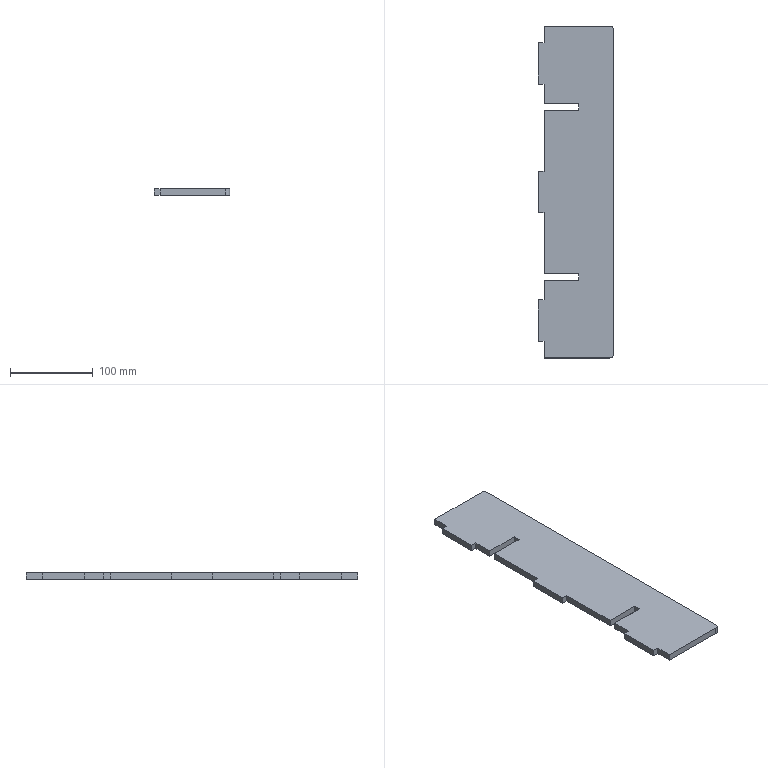Part | SolidWorks | features FlatPattern 1, SMBaseFlange 1, SheetMetal 1 | 1 solid | 28 faces | box 91 x 400 x 8 mm | volume 271738 mm3 | plane 26 | cylinder 2 | commonest cylinder face diameters 10 x2
STEP:
#1=CARTESIAN_POINT('',(598.509,-204.15,0.));
#2=VERTEX_POINT('',#1);
#3=CARTESIAN_POINT('',(598.509,-224.15,0.));
#4=VERTEX_POINT('',#3);
#5=CARTESIAN_POINT('',(598.509,-204.15,0.));
#6=DIRECTION('',(0.,-1.,0.));
#7=VECTOR('',#6,1000.);
#8=LINE('',#5,#7);
#9=EDGE_CURVE('',#2,#4,#8,.T.);
#10=ORIENTED_EDGE('',*,*,#9,.F.);
#11=CARTESIAN_POINT('',(598.509,-204.15,-8.));
#12=VERTEX_POINT('',#11);
#13=CARTESIAN_POINT('',(598.509,-204.15,-8.));
#14=DIRECTION('',(0.,0.,1.));
#15=VECTOR('',#14,1000.);
#16=LINE('',#13,#15);
#17=EDGE_CURVE('',#12,#2,#16,.T.);
#18=ORIENTED_EDGE('',*,*,#17,.F.);
#19=CARTESIAN_POINT('',(598.509,-224.15,-8.));
#20=VERTEX_POINT('',#19);
#21=CARTESIAN_POINT('',(598.509,-204.15,-8.));
#22=DIRECTION('',(0.,-1.,0.));
#23=VECTOR('',#22,1000.);
#24=LINE('',#21,#23);
#25=EDGE_CURVE('',#12,#20,#24,.T.);
#26=ORIENTED_EDGE('',*,*,#25,.T.);
#27=CARTESIAN_POINT('',(598.509,-224.15,-8.));
#28=DIRECTION('',(0.,0.,1.));
#29=VECTOR('',#28,1000.);
#30=LINE('',#27,#29);
#31=EDGE_CURVE('',#20,#4,#30,.T.);
#32=ORIENTED_EDGE('',*,*,#31,.T.);
#33=EDGE_LOOP('',(#10,#18,#26,#32));
#34=FACE_OUTER_BOUND('',#33,.T.);
#35=CARTESIAN_POINT('',(598.509,-204.15,-8.));
#36=DIRECTION('',(-1.,0.,0.));
#37=DIRECTION('',(0.,0.,1.));
#38=AXIS2_PLACEMENT_3D('',#35,#36,#37);
#39=PLANE('',#38);
#40=ADVANCED_FACE('',(#34),#39,.T.);
#41=CARTESIAN_POINT('',(591.509,-204.15,0.));
#42=VERTEX_POINT('',#41);
#43=CARTESIAN_POINT('',(591.509,-204.15,0.));
#44=DIRECTION('',(1.,0.,0.));
#45=VECTOR('',#44,1000.);
#46=LINE('',#43,#45);
#47=EDGE_CURVE('',#42,#2,#46,.T.);
#48=ORIENTED_EDGE('',*,*,#47,.F.);
#49=CARTESIAN_POINT('',(591.509,-204.15,-8.));
#50=VERTEX_POINT('',#49);
#51=CARTESIAN_POINT('',(591.509,-204.15,-8.));
#52=DIRECTION('',(0.,0.,1.));
#53=VECTOR('',#52,1000.);
#54=LINE('',#51,#53);
#55=EDGE_CURVE('',#50,#42,#54,.T.);
#56=ORIENTED_EDGE('',*,*,#55,.F.);
#57=CARTESIAN_POINT('',(591.509,-204.15,-8.));
#58=DIRECTION('',(1.,0.,0.));
#59=VECTOR('',#58,1000.);
#60=LINE('',#57,#59);
#61=EDGE_CURVE('',#50,#12,#60,.T.);
#62=ORIENTED_EDGE('',*,*,#61,.T.);
#63=ORIENTED_EDGE('',*,*,#17,.T.);
#64=EDGE_LOOP('',(#48,#56,#62,#63));
#65=FACE_OUTER_BOUND('',#64,.T.);
#66=CARTESIAN_POINT('',(591.509,-204.15,-8.));
#67=DIRECTION('',(0.,-1.,0.));
#68=DIRECTION('',(1.,0.,0.));
#69=AXIS2_PLACEMENT_3D('',#66,#67,#68);
#70=PLANE('',#69);
#71=ADVANCED_FACE('',(#65),#70,.T.);
#72=CARTESIAN_POINT('',(591.509,-154.15,0.));
#73=VERTEX_POINT('',#72);
#74=CARTESIAN_POINT('',(591.509,-154.15,0.));
#75=DIRECTION('',(0.,-1.,0.));
#76=VECTOR('',#75,1000.);
#77=LINE('',#74,#76);
#78=EDGE_CURVE('',#73,#42,#77,.T.);
#79=ORIENTED_EDGE('',*,*,#78,.F.);
#80=CARTESIAN_POINT('',(591.509,-154.15,-8.));
#81=VERTEX_POINT('',#80);
#82=CARTESIAN_POINT('',(591.509,-154.15,-8.));
#83=DIRECTION('',(0.,0.,1.));
#84=VECTOR('',#83,1000.);
#85=LINE('',#82,#84);
#86=EDGE_CURVE('',#81,#73,#85,.T.);
#87=ORIENTED_EDGE('',*,*,#86,.F.);
#88=CARTESIAN_POINT('',(591.509,-154.15,-8.));
#89=DIRECTION('',(0.,-1.,0.));
#90=VECTOR('',#89,1000.);
#91=LINE('',#88,#90);
#92=EDGE_CURVE('',#81,#50,#91,.T.);
#93=ORIENTED_EDGE('',*,*,#92,.T.);
#94=ORIENTED_EDGE('',*,*,#55,.T.);
#95=EDGE_LOOP('',(#79,#87,#93,#94));
#96=FACE_OUTER_BOUND('',#95,.T.);
#97=CARTESIAN_POINT('',(591.509,-154.15,-8.));
#98=DIRECTION('',(-1.,0.,0.));
#99=DIRECTION('',(0.,0.,1.));
#100=AXIS2_PLACEMENT_3D('',#97,#98,#99);
#101=PLANE('',#100);
#102=ADVANCED_FACE('',(#96),#101,.T.);
#103=CARTESIAN_POINT('',(598.509,-154.15,0.));
#104=VERTEX_POINT('',#103);
#105=CARTESIAN_POINT('',(598.509,-154.15,0.));
#106=DIRECTION('',(-1.,0.,0.));
#107=VECTOR('',#106,1000.);
#108=LINE('',#105,#107);
#109=EDGE_CURVE('',#104,#73,#108,.T.);
#110=ORIENTED_EDGE('',*,*,#109,.F.);
#111=CARTESIAN_POINT('',(598.509,-154.15,-8.));
#112=VERTEX_POINT('',#111);
#113=CARTESIAN_POINT('',(598.509,-154.15,-8.));
#114=DIRECTION('',(0.,0.,1.));
#115=VECTOR('',#114,1000.);
#116=LINE('',#113,#115);
#117=EDGE_CURVE('',#112,#104,#116,.T.);
#118=ORIENTED_EDGE('',*,*,#117,.F.);
#119=CARTESIAN_POINT('',(598.509,-154.15,-8.));
#120=DIRECTION('',(-1.,0.,0.));
#121=VECTOR('',#120,1000.);
#122=LINE('',#119,#121);
#123=EDGE_CURVE('',#112,#81,#122,.T.);
#124=ORIENTED_EDGE('',*,*,#123,.T.);
#125=ORIENTED_EDGE('',*,*,#86,.T.);
#126=EDGE_LOOP('',(#110,#118,#124,#125));
#127=FACE_OUTER_BOUND('',#126,.T.);
#128=CARTESIAN_POINT('',(598.509,-154.15,-8.));
#129=DIRECTION('',(0.,1.,0.));
#130=DIRECTION('',(-1.,0.,0.));
#131=AXIS2_PLACEMENT_3D('',#128,#129,#130);
#132=PLANE('',#131);
#133=ADVANCED_FACE('',(#127),#132,.T.);
#134=CARTESIAN_POINT('',(598.509,-130.65,0.));
#135=VERTEX_POINT('',#134);
#136=CARTESIAN_POINT('',(598.509,-130.65,0.));
#137=DIRECTION('',(0.,-1.,0.));
#138=VECTOR('',#137,1000.);
#139=LINE('',#136,#138);
#140=EDGE_CURVE('',#135,#104,#139,.T.);
#141=ORIENTED_EDGE('',*,*,#140,.F.);
#142=CARTESIAN_POINT('',(598.509,-130.65,-8.));
#143=VERTEX_POINT('',#142);
#144=CARTESIAN_POINT('',(598.509,-130.65,-8.));
#145=DIRECTION('',(0.,0.,1.));
#146=VECTOR('',#145,1000.);
#147=LINE('',#144,#146);
#148=EDGE_CURVE('',#143,#135,#147,.T.);
#149=ORIENTED_EDGE('',*,*,#148,.F.);
#150=CARTESIAN_POINT('',(598.509,-130.65,-8.));
#151=DIRECTION('',(0.,-1.,0.));
#152=VECTOR('',#151,1000.);
#153=LINE('',#150,#152);
#154=EDGE_CURVE('',#143,#112,#153,.T.);
#155=ORIENTED_EDGE('',*,*,#154,.T.);
#156=ORIENTED_EDGE('',*,*,#117,.T.);
#157=EDGE_LOOP('',(#141,#149,#155,#156));
#158=FACE_OUTER_BOUND('',#157,.T.);
#159=CARTESIAN_POINT('',(598.509,-130.65,-8.));
#160=DIRECTION('',(-1.,0.,0.));
#161=DIRECTION('',(0.,-1.,0.));
#162=AXIS2_PLACEMENT_3D('',#159,#160,#161);
#163=PLANE('',#162);
#164=ADVANCED_FACE('',(#158),#163,.T.);
#165=CARTESIAN_POINT('',(640.509,-130.65,0.));
#166=VERTEX_POINT('',#165);
#167=CARTESIAN_POINT('',(640.509,-130.65,0.));
#168=DIRECTION('',(-1.,0.,0.));
#169=VECTOR('',#168,1000.);
#170=LINE('',#167,#169);
#171=EDGE_CURVE('',#166,#135,#170,.T.);
#172=ORIENTED_EDGE('',*,*,#171,.F.);
#173=CARTESIAN_POINT('',(640.509,-130.65,-8.));
#174=VERTEX_POINT('',#173);
#175=CARTESIAN_POINT('',(640.509,-130.65,-8.));
#176=DIRECTION('',(0.,0.,1.));
#177=VECTOR('',#176,1000.);
#178=LINE('',#175,#177);
#179=EDGE_CURVE('',#174,#166,#178,.T.);
#180=ORIENTED_EDGE('',*,*,#179,.F.);
#181=CARTESIAN_POINT('',(640.509,-130.65,-8.));
#182=DIRECTION('',(-1.,0.,0.));
#183=VECTOR('',#182,1000.);
#184=LINE('',#181,#183);
#185=EDGE_CURVE('',#174,#143,#184,.T.);
#186=ORIENTED_EDGE('',*,*,#185,.T.);
#187=ORIENTED_EDGE('',*,*,#148,.T.);
#188=EDGE_LOOP('',(#172,#180,#186,#187));
#189=FACE_OUTER_BOUND('',#188,.T.);
#190=CARTESIAN_POINT('',(640.509,-130.65,-8.));
#191=DIRECTION('',(0.,1.,0.));
#192=DIRECTION('',(-1.,0.,0.));
#193=AXIS2_PLACEMENT_3D('',#190,#191,#192);
#194=PLANE('',#193);
#195=ADVANCED_FACE('',(#189),#194,.T.);
#196=CARTESIAN_POINT('',(640.509,-122.65,0.));
#197=VERTEX_POINT('',#196);
#198=CARTESIAN_POINT('',(640.509,-122.65,0.));
#199=DIRECTION('',(0.,-1.,0.));
#200=VECTOR('',#199,1000.);
#201=LINE('',#198,#200);
#202=EDGE_CURVE('',#197,#166,#201,.T.);
#203=ORIENTED_EDGE('',*,*,#202,.F.);
#204=CARTESIAN_POINT('',(640.509,-122.65,-8.));
#205=VERTEX_POINT('',#204);
#206=CARTESIAN_POINT('',(640.509,-122.65,-8.));
#207=DIRECTION('',(0.,0.,1.));
#208=VECTOR('',#207,1000.);
#209=LINE('',#206,#208);
#210=EDGE_CURVE('',#205,#197,#209,.T.);
#211=ORIENTED_EDGE('',*,*,#210,.F.);
#212=CARTESIAN_POINT('',(640.509,-122.65,-8.));
#213=DIRECTION('',(0.,-1.,0.));
#214=VECTOR('',#213,1000.);
#215=LINE('',#212,#214);
#216=EDGE_CURVE('',#205,#174,#215,.T.);
#217=ORIENTED_EDGE('',*,*,#216,.T.);
#218=ORIENTED_EDGE('',*,*,#179,.T.);
#219=EDGE_LOOP('',(#203,#211,#217,#218));
#220=FACE_OUTER_BOUND('',#219,.T.);
#221=CARTESIAN_POINT('',(640.509,-122.65,-8.));
#222=DIRECTION('',(-1.,0.,0.));
#223=DIRECTION('',(0.,0.,1.));
#224=AXIS2_PLACEMENT_3D('',#221,#222,#223);
#225=PLANE('',#224);
#226=ADVANCED_FACE('',(#220),#225,.T.);
#227=CARTESIAN_POINT('',(598.509,-122.65,0.));
#228=VERTEX_POINT('',#227);
#229=CARTESIAN_POINT('',(598.509,-122.65,0.));
#230=DIRECTION('',(1.,0.,0.));
#231=VECTOR('',#230,1000.);
#232=LINE('',#229,#231);
#233=EDGE_CURVE('',#228,#197,#232,.T.);
#234=ORIENTED_EDGE('',*,*,#233,.F.);
#235=CARTESIAN_POINT('',(598.509,-122.65,-8.));
#236=VERTEX_POINT('',#235);
#237=CARTESIAN_POINT('',(598.509,-122.65,-8.));
#238=DIRECTION('',(0.,0.,1.));
#239=VECTOR('',#238,1000.);
#240=LINE('',#237,#239);
#241=EDGE_CURVE('',#236,#228,#240,.T.);
#242=ORIENTED_EDGE('',*,*,#241,.F.);
#243=CARTESIAN_POINT('',(598.509,-122.65,-8.));
#244=DIRECTION('',(1.,0.,0.));
#245=VECTOR('',#244,1000.);
#246=LINE('',#243,#245);
#247=EDGE_CURVE('',#236,#205,#246,.T.);
#248=ORIENTED_EDGE('',*,*,#247,.T.);
#249=ORIENTED_EDGE('',*,*,#210,.T.);
#250=EDGE_LOOP('',(#234,#242,#248,#249));
#251=FACE_OUTER_BOUND('',#250,.T.);
#252=CARTESIAN_POINT('',(598.509,-122.65,-8.));
#253=DIRECTION('',(0.,-1.,0.));
#254=DIRECTION('',(1.,0.,0.));
#255=AXIS2_PLACEMENT_3D('',#252,#253,#254);
#256=PLANE('',#255);
#257=ADVANCED_FACE('',(#251),#256,.T.);
#258=CARTESIAN_POINT('',(598.509,-49.15,0.));
#259=VERTEX_POINT('',#258);
#260=CARTESIAN_POINT('',(598.509,-49.15,0.));
#261=DIRECTION('',(0.,-1.,0.));
#262=VECTOR('',#261,1000.);
#263=LINE('',#260,#262);
#264=EDGE_CURVE('',#259,#228,#263,.T.);
#265=ORIENTED_EDGE('',*,*,#264,.F.);
#266=CARTESIAN_POINT('',(598.509,-49.15,-8.));
#267=VERTEX_POINT('',#266);
#268=CARTESIAN_POINT('',(598.509,-49.15,-8.));
#269=DIRECTION('',(0.,0.,1.));
#270=VECTOR('',#269,1000.);
#271=LINE('',#268,#270);
#272=EDGE_CURVE('',#267,#259,#271,.T.);
#273=ORIENTED_EDGE('',*,*,#272,.F.);
#274=CARTESIAN_POINT('',(598.509,-49.15,-8.));
#275=DIRECTION('',(0.,-1.,0.));
#276=VECTOR('',#275,1000.);
#277=LINE('',#274,#276);
#278=EDGE_CURVE('',#267,#236,#277,.T.);
#279=ORIENTED_EDGE('',*,*,#278,.T.);
#280=ORIENTED_EDGE('',*,*,#241,.T.);
#281=EDGE_LOOP('',(#265,#273,#279,#280));
#282=FACE_OUTER_BOUND('',#281,.T.);
#283=CARTESIAN_POINT('',(598.509,-49.15,-8.));
#284=DIRECTION('',(-1.,0.,0.));
#285=DIRECTION('',(0.,-1.,0.));
#286=AXIS2_PLACEMENT_3D('',#283,#284,#285);
#287=PLANE('',#286);
#288=ADVANCED_FACE('',(#282),#287,.T.);
#289=CARTESIAN_POINT('',(591.509,-49.15,0.));
#290=VERTEX_POINT('',#289);
#291=CARTESIAN_POINT('',(591.509,-49.15,0.));
#292=DIRECTION('',(1.,0.,0.));
#293=VECTOR('',#292,1000.);
#294=LINE('',#291,#293);
#295=EDGE_CURVE('',#290,#259,#294,.T.);
#296=ORIENTED_EDGE('',*,*,#295,.F.);
#297=CARTESIAN_POINT('',(591.509,-49.15,-8.));
#298=VERTEX_POINT('',#297);
#299=CARTESIAN_POINT('',(591.509,-49.15,-8.));
#300=DIRECTION('',(0.,0.,1.));
#301=VECTOR('',#300,1000.);
#302=LINE('',#299,#301);
#303=EDGE_CURVE('',#298,#290,#302,.T.);
#304=ORIENTED_EDGE('',*,*,#303,.F.);
#305=CARTESIAN_POINT('',(591.509,-49.15,-8.));
#306=DIRECTION('',(1.,0.,0.));
#307=VECTOR('',#306,1000.);
#308=LINE('',#305,#307);
#309=EDGE_CURVE('',#298,#267,#308,.T.);
#310=ORIENTED_EDGE('',*,*,#309,.T.);
#311=ORIENTED_EDGE('',*,*,#272,.T.);
#312=EDGE_LOOP('',(#296,#304,#310,#311));
#313=FACE_OUTER_BOUND('',#312,.T.);
#314=CARTESIAN_POINT('',(591.509,-49.15,-8.));
#315=DIRECTION('',(0.,-1.,0.));
#316=DIRECTION('',(1.,0.,0.));
#317=AXIS2_PLACEMENT_3D('',#314,#315,#316);
#318=PLANE('',#317);
#319=ADVANCED_FACE('',(#313),#318,.T.);
#320=CARTESIAN_POINT('',(591.509,0.8496,0.));
#321=VERTEX_POINT('',#320);
#322=CARTESIAN_POINT('',(591.509,0.8496,0.));
#323=DIRECTION('',(0.,-1.,0.));
#324=VECTOR('',#323,1000.);
#325=LINE('',#322,#324);
#326=EDGE_CURVE('',#321,#290,#325,.T.);
#327=ORIENTED_EDGE('',*,*,#326,.F.);
#328=CARTESIAN_POINT('',(591.509,0.8496,-8.));
#329=VERTEX_POINT('',#328);
#330=CARTESIAN_POINT('',(591.509,0.8496,-8.));
#331=DIRECTION('',(0.,0.,1.));
#332=VECTOR('',#331,1000.);
#333=LINE('',#330,#332);
#334=EDGE_CURVE('',#329,#321,#333,.T.);
#335=ORIENTED_EDGE('',*,*,#334,.F.);
#336=CARTESIAN_POINT('',(591.509,0.8496,-8.));
#337=DIRECTION('',(0.,-1.,0.));
#338=VECTOR('',#337,1000.);
#339=LINE('',#336,#338);
#340=EDGE_CURVE('',#329,#298,#339,.T.);
#341=ORIENTED_EDGE('',*,*,#340,.T.);
#342=ORIENTED_EDGE('',*,*,#303,.T.);
#343=EDGE_LOOP('',(#327,#335,#341,#342));
#344=FACE_OUTER_BOUND('',#343,.T.);
#345=CARTESIAN_POINT('',(591.509,0.8496,-8.));
#346=DIRECTION('',(-1.,0.,0.));
#347=DIRECTION('',(0.,0.,1.));
#348=AXIS2_PLACEMENT_3D('',#345,#346,#347);
#349=PLANE('',#348);
#350=ADVANCED_FACE('',(#344),#349,.T.);
#351=CARTESIAN_POINT('',(598.509,0.8496,0.));
#352=VERTEX_POINT('',#351);
#353=CARTESIAN_POINT('',(598.509,0.8496,0.));
#354=DIRECTION('',(-1.,0.,0.));
#355=VECTOR('',#354,1000.);
#356=LINE('',#353,#355);
#357=EDGE_CURVE('',#352,#321,#356,.T.);
#358=ORIENTED_EDGE('',*,*,#357,.F.);
#359=CARTESIAN_POINT('',(598.509,0.8496,-8.));
#360=VERTEX_POINT('',#359);
#361=CARTESIAN_POINT('',(598.509,0.8496,-8.));
#362=DIRECTION('',(0.,0.,1.));
#363=VECTOR('',#362,1000.);
#364=LINE('',#361,#363);
#365=EDGE_CURVE('',#360,#352,#364,.T.);
#366=ORIENTED_EDGE('',*,*,#365,.F.);
#367=CARTESIAN_POINT('',(598.509,0.8496,-8.));
#368=DIRECTION('',(-1.,0.,0.));
#369=VECTOR('',#368,1000.);
#370=LINE('',#367,#369);
#371=EDGE_CURVE('',#360,#329,#370,.T.);
#372=ORIENTED_EDGE('',*,*,#371,.T.);
#373=ORIENTED_EDGE('',*,*,#334,.T.);
#374=EDGE_LOOP('',(#358,#366,#372,#373));
#375=FACE_OUTER_BOUND('',#374,.T.);
#376=CARTESIAN_POINT('',(598.509,0.8496,-8.));
#377=DIRECTION('',(0.,1.,0.));
#378=DIRECTION('',(0.,0.,1.));
#379=AXIS2_PLACEMENT_3D('',#376,#377,#378);
#380=PLANE('',#379);
#381=ADVANCED_FACE('',(#375),#380,.T.);
#382=CARTESIAN_POINT('',(598.509,74.35,0.));
#383=VERTEX_POINT('',#382);
#384=CARTESIAN_POINT('',(598.509,74.35,0.));
#385=DIRECTION('',(0.,-1.,0.));
#386=VECTOR('',#385,1000.);
#387=LINE('',#384,#386);
#388=EDGE_CURVE('',#383,#352,#387,.T.);
#389=ORIENTED_EDGE('',*,*,#388,.F.);
#390=CARTESIAN_POINT('',(598.509,74.35,-8.));
#391=VERTEX_POINT('',#390);
#392=CARTESIAN_POINT('',(598.509,74.35,-8.));
#393=DIRECTION('',(0.,0.,1.));
#394=VECTOR('',#393,1000.);
#395=LINE('',#392,#394);
#396=EDGE_CURVE('',#391,#383,#395,.T.);
#397=ORIENTED_EDGE('',*,*,#396,.F.);
#398=CARTESIAN_POINT('',(598.509,74.35,-8.));
#399=DIRECTION('',(0.,-1.,0.));
#400=VECTOR('',#399,1000.);
#401=LINE('',#398,#400);
#402=EDGE_CURVE('',#391,#360,#401,.T.);
#403=ORIENTED_EDGE('',*,*,#402,.T.);
#404=ORIENTED_EDGE('',*,*,#365,.T.);
#405=EDGE_LOOP('',(#389,#397,#403,#404));
#406=FACE_OUTER_BOUND('',#405,.T.);
#407=CARTESIAN_POINT('',(598.509,74.35,-8.));
#408=DIRECTION('',(-1.,0.,0.));
#409=DIRECTION('',(0.,-1.,0.));
#410=AXIS2_PLACEMENT_3D('',#407,#408,#409);
#411=PLANE('',#410);
#412=ADVANCED_FACE('',(#406),#411,.T.);
#413=CARTESIAN_POINT('',(640.509,74.35,0.));
#414=VERTEX_POINT('',#413);
#415=CARTESIAN_POINT('',(640.509,74.35,0.));
#416=DIRECTION('',(-1.,0.,0.));
#417=VECTOR('',#416,1000.);
#418=LINE('',#415,#417);
#419=EDGE_CURVE('',#414,#383,#418,.T.);
#420=ORIENTED_EDGE('',*,*,#419,.F.);
#421=CARTESIAN_POINT('',(640.509,74.35,-8.));
#422=VERTEX_POINT('',#421);
#423=CARTESIAN_POINT('',(640.509,74.35,-8.));
#424=DIRECTION('',(0.,0.,1.));
#425=VECTOR('',#424,1000.);
#426=LINE('',#423,#425);
#427=EDGE_CURVE('',#422,#414,#426,.T.);
#428=ORIENTED_EDGE('',*,*,#427,.F.);
#429=CARTESIAN_POINT('',(640.509,74.35,-8.));
#430=DIRECTION('',(-1.,0.,0.));
#431=VECTOR('',#430,1000.);
#432=LINE('',#429,#431);
#433=EDGE_CURVE('',#422,#391,#432,.T.);
#434=ORIENTED_EDGE('',*,*,#433,.T.);
#435=ORIENTED_EDGE('',*,*,#396,.T.);
#436=EDGE_LOOP('',(#420,#428,#434,#435));
#437=FACE_OUTER_BOUND('',#436,.T.);
#438=CARTESIAN_POINT('',(640.509,74.35,-8.));
#439=DIRECTION('',(0.,1.,0.));
#440=DIRECTION('',(0.,0.,1.));
#441=AXIS2_PLACEMENT_3D('',#438,#439,#440);
#442=PLANE('',#441);
#443=ADVANCED_FACE('',(#437),#442,.T.);
#444=CARTESIAN_POINT('',(640.509,82.35,0.));
#445=VERTEX_POINT('',#444);
#446=CARTESIAN_POINT('',(640.509,82.35,0.));
#447=DIRECTION('',(0.,-1.,0.));
#448=VECTOR('',#447,1000.);
#449=LINE('',#446,#448);
#450=EDGE_CURVE('',#445,#414,#449,.T.);
#451=ORIENTED_EDGE('',*,*,#450,.F.);
#452=CARTESIAN_POINT('',(640.509,82.35,-8.));
#453=VERTEX_POINT('',#452);
#454=CARTESIAN_POINT('',(640.509,82.35,-8.));
#455=DIRECTION('',(0.,0.,1.));
#456=VECTOR('',#455,1000.);
#457=LINE('',#454,#456);
#458=EDGE_CURVE('',#453,#445,#457,.T.);
#459=ORIENTED_EDGE('',*,*,#458,.F.);
#460=CARTESIAN_POINT('',(640.509,82.35,-8.));
#461=DIRECTION('',(0.,-1.,0.));
#462=VECTOR('',#461,1000.);
#463=LINE('',#460,#462);
#464=EDGE_CURVE('',#453,#422,#463,.T.);
#465=ORIENTED_EDGE('',*,*,#464,.T.);
#466=ORIENTED_EDGE('',*,*,#427,.T.);
#467=EDGE_LOOP('',(#451,#459,#465,#466));
#468=FACE_OUTER_BOUND('',#467,.T.);
#469=CARTESIAN_POINT('',(640.509,82.35,-8.));
#470=DIRECTION('',(-1.,0.,0.));
#471=DIRECTION('',(0.,0.,1.));
#472=AXIS2_PLACEMENT_3D('',#469,#470,#471);
#473=PLANE('',#472);
#474=ADVANCED_FACE('',(#468),#473,.T.);
#475=CARTESIAN_POINT('',(598.509,82.35,0.));
#476=VERTEX_POINT('',#475);
#477=CARTESIAN_POINT('',(598.509,82.35,0.));
#478=DIRECTION('',(1.,0.,0.));
#479=VECTOR('',#478,1000.);
#480=LINE('',#477,#479);
#481=EDGE_CURVE('',#476,#445,#480,.T.);
#482=ORIENTED_EDGE('',*,*,#481,.F.);
#483=CARTESIAN_POINT('',(598.509,82.35,-8.));
#484=VERTEX_POINT('',#483);
#485=CARTESIAN_POINT('',(598.509,82.35,-8.));
#486=DIRECTION('',(0.,0.,1.));
#487=VECTOR('',#486,1000.);
#488=LINE('',#485,#487);
#489=EDGE_CURVE('',#484,#476,#488,.T.);
#490=ORIENTED_EDGE('',*,*,#489,.F.);
#491=CARTESIAN_POINT('',(598.509,82.35,-8.));
#492=DIRECTION('',(1.,0.,0.));
#493=VECTOR('',#492,1000.);
#494=LINE('',#491,#493);
#495=EDGE_CURVE('',#484,#453,#494,.T.);
#496=ORIENTED_EDGE('',*,*,#495,.T.);
#497=ORIENTED_EDGE('',*,*,#458,.T.);
#498=EDGE_LOOP('',(#482,#490,#496,#497));
#499=FACE_OUTER_BOUND('',#498,.T.);
#500=CARTESIAN_POINT('',(598.509,82.35,-8.));
#501=DIRECTION('',(0.,-1.,0.));
#502=DIRECTION('',(0.,0.,-1.));
#503=AXIS2_PLACEMENT_3D('',#500,#501,#502);
#504=PLANE('',#503);
#505=ADVANCED_FACE('',(#499),#504,.T.);
#506=CARTESIAN_POINT('',(598.509,105.85,0.));
#507=VERTEX_POINT('',#506);
#508=CARTESIAN_POINT('',(598.509,105.85,0.));
#509=DIRECTION('',(0.,-1.,0.));
#510=VECTOR('',#509,1000.);
#511=LINE('',#508,#510);
#512=EDGE_CURVE('',#507,#476,#511,.T.);
#513=ORIENTED_EDGE('',*,*,#512,.F.);
#514=CARTESIAN_POINT('',(598.509,105.85,-8.));
#515=VERTEX_POINT('',#514);
#516=CARTESIAN_POINT('',(598.509,105.85,-8.));
#517=DIRECTION('',(0.,0.,1.));
#518=VECTOR('',#517,1000.);
#519=LINE('',#516,#518);
#520=EDGE_CURVE('',#515,#507,#519,.T.);
#521=ORIENTED_EDGE('',*,*,#520,.F.);
#522=CARTESIAN_POINT('',(598.509,105.85,-8.));
#523=DIRECTION('',(0.,-1.,0.));
#524=VECTOR('',#523,1000.);
#525=LINE('',#522,#524);
#526=EDGE_CURVE('',#515,#484,#525,.T.);
#527=ORIENTED_EDGE('',*,*,#526,.T.);
#528=ORIENTED_EDGE('',*,*,#489,.T.);
#529=EDGE_LOOP('',(#513,#521,#527,#528));
#530=FACE_OUTER_BOUND('',#529,.T.);
#531=CARTESIAN_POINT('',(598.509,105.85,-8.));
#532=DIRECTION('',(-1.,0.,0.));
#533=DIRECTION('',(0.,-1.,0.));
#534=AXIS2_PLACEMENT_3D('',#531,#532,#533);
#535=PLANE('',#534);
#536=ADVANCED_FACE('',(#530),#535,.T.);
#537=CARTESIAN_POINT('',(591.509,105.85,0.));
#538=VERTEX_POINT('',#537);
#539=CARTESIAN_POINT('',(591.509,105.85,0.));
#540=DIRECTION('',(1.,0.,0.));
#541=VECTOR('',#540,1000.);
#542=LINE('',#539,#541);
#543=EDGE_CURVE('',#538,#507,#542,.T.);
#544=ORIENTED_EDGE('',*,*,#543,.F.);
#545=CARTESIAN_POINT('',(591.509,105.85,-8.));
#546=VERTEX_POINT('',#545);
#547=CARTESIAN_POINT('',(591.509,105.85,-8.));
#548=DIRECTION('',(0.,0.,1.));
#549=VECTOR('',#548,1000.);
#550=LINE('',#547,#549);
#551=EDGE_CURVE('',#546,#538,#550,.T.);
#552=ORIENTED_EDGE('',*,*,#551,.F.);
#553=CARTESIAN_POINT('',(591.509,105.85,-8.));
#554=DIRECTION('',(1.,0.,0.));
#555=VECTOR('',#554,1000.);
#556=LINE('',#553,#555);
#557=EDGE_CURVE('',#546,#515,#556,.T.);
#558=ORIENTED_EDGE('',*,*,#557,.T.);
#559=ORIENTED_EDGE('',*,*,#520,.T.);
#560=EDGE_LOOP('',(#544,#552,#558,#559));
#561=FACE_OUTER_BOUND('',#560,.T.);
#562=CARTESIAN_POINT('',(591.509,105.85,-8.));
#563=DIRECTION('',(0.,-1.,0.));
#564=DIRECTION('',(1.,0.,0.));
#565=AXIS2_PLACEMENT_3D('',#562,#563,#564);
#566=PLANE('',#565);
#567=ADVANCED_FACE('',(#561),#566,.T.);
#568=CARTESIAN_POINT('',(591.509,155.85,0.));
#569=VERTEX_POINT('',#568);
#570=CARTESIAN_POINT('',(591.509,155.85,0.));
#571=DIRECTION('',(0.,-1.,0.));
#572=VECTOR('',#571,1000.);
#573=LINE('',#570,#572);
#574=EDGE_CURVE('',#569,#538,#573,.T.);
#575=ORIENTED_EDGE('',*,*,#574,.F.);
#576=CARTESIAN_POINT('',(591.509,155.85,-8.));
#577=VERTEX_POINT('',#576);
#578=CARTESIAN_POINT('',(591.509,155.85,-8.));
#579=DIRECTION('',(0.,0.,1.));
#580=VECTOR('',#579,1000.);
#581=LINE('',#578,#580);
#582=EDGE_CURVE('',#577,#569,#581,.T.);
#583=ORIENTED_EDGE('',*,*,#582,.F.);
#584=CARTESIAN_POINT('',(591.509,155.85,-8.));
#585=DIRECTION('',(0.,-1.,0.));
#586=VECTOR('',#585,1000.);
#587=LINE('',#584,#586);
#588=EDGE_CURVE('',#577,#546,#587,.T.);
#589=ORIENTED_EDGE('',*,*,#588,.T.);
#590=ORIENTED_EDGE('',*,*,#551,.T.);
#591=EDGE_LOOP('',(#575,#583,#589,#590));
#592=FACE_OUTER_BOUND('',#591,.T.);
#593=CARTESIAN_POINT('',(591.509,155.85,-8.));
#594=DIRECTION('',(-1.,0.,0.));
#595=DIRECTION('',(0.,0.,1.));
#596=AXIS2_PLACEMENT_3D('',#593,#594,#595);
#597=PLANE('',#596);
#598=ADVANCED_FACE('',(#592),#597,.T.);
#599=CARTESIAN_POINT('',(598.509,155.85,0.));
#600=VERTEX_POINT('',#599);
#601=CARTESIAN_POINT('',(598.509,155.85,0.));
#602=DIRECTION('',(-1.,0.,0.));
#603=VECTOR('',#602,1000.);
#604=LINE('',#601,#603);
#605=EDGE_CURVE('',#600,#569,#604,.T.);
#606=ORIENTED_EDGE('',*,*,#605,.F.);
#607=CARTESIAN_POINT('',(598.509,155.85,-8.));
#608=VERTEX_POINT('',#607);
#609=CARTESIAN_POINT('',(598.509,155.85,-8.));
#610=DIRECTION('',(0.,0.,1.));
#611=VECTOR('',#610,1000.);
#612=LINE('',#609,#611);
#613=EDGE_CURVE('',#608,#600,#612,.T.);
#614=ORIENTED_EDGE('',*,*,#613,.F.);
#615=CARTESIAN_POINT('',(598.509,155.85,-8.));
#616=DIRECTION('',(-1.,0.,0.));
#617=VECTOR('',#616,1000.);
#618=LINE('',#615,#617);
#619=EDGE_CURVE('',#608,#577,#618,.T.);
#620=ORIENTED_EDGE('',*,*,#619,.T.);
#621=ORIENTED_EDGE('',*,*,#582,.T.);
#622=EDGE_LOOP('',(#606,#614,#620,#621));
#623=FACE_OUTER_BOUND('',#622,.T.);
#624=CARTESIAN_POINT('',(598.509,155.85,-8.));
#625=DIRECTION('',(0.,1.,0.));
#626=DIRECTION('',(0.,0.,1.));
#627=AXIS2_PLACEMENT_3D('',#624,#625,#626);
#628=PLANE('',#627);
#629=ADVANCED_FACE('',(#623),#628,.T.);
#630=CARTESIAN_POINT('',(598.509,175.85,0.));
#631=VERTEX_POINT('',#630);
#632=CARTESIAN_POINT('',(598.509,175.85,0.));
#633=DIRECTION('',(0.,-1.,0.));
#634=VECTOR('',#633,1000.);
#635=LINE('',#632,#634);
#636=EDGE_CURVE('',#631,#600,#635,.T.);
#637=ORIENTED_EDGE('',*,*,#636,.F.);
#638=CARTESIAN_POINT('',(598.509,175.85,-8.));
#639=VERTEX_POINT('',#638);
#640=CARTESIAN_POINT('',(598.509,175.85,-8.));
#641=DIRECTION('',(0.,0.,1.));
#642=VECTOR('',#641,1000.);
#643=LINE('',#640,#642);
#644=EDGE_CURVE('',#639,#631,#643,.T.);
#645=ORIENTED_EDGE('',*,*,#644,.F.);
#646=CARTESIAN_POINT('',(598.509,175.85,-8.));
#647=DIRECTION('',(0.,-1.,0.));
#648=VECTOR('',#647,1000.);
#649=LINE('',#646,#648);
#650=EDGE_CURVE('',#639,#608,#649,.T.);
#651=ORIENTED_EDGE('',*,*,#650,.T.);
#652=ORIENTED_EDGE('',*,*,#613,.T.);
#653=EDGE_LOOP('',(#637,#645,#651,#652));
#654=FACE_OUTER_BOUND('',#653,.T.);
#655=CARTESIAN_POINT('',(598.509,175.85,-8.));
#656=DIRECTION('',(-1.,0.,0.));
#657=DIRECTION('',(0.,0.,1.));
#658=AXIS2_PLACEMENT_3D('',#655,#656,#657);
#659=PLANE('',#658);
#660=ADVANCED_FACE('',(#654),#659,.T.);
#661=CARTESIAN_POINT('',(677.509,175.85,0.));
#662=VERTEX_POINT('',#661);
#663=CARTESIAN_POINT('',(677.509,175.85,0.));
#664=DIRECTION('',(-1.,0.,0.));
#665=VECTOR('',#664,1000.);
#666=LINE('',#663,#665);
#667=EDGE_CURVE('',#662,#631,#666,.T.);
#668=ORIENTED_EDGE('',*,*,#667,.F.);
#669=CARTESIAN_POINT('',(677.509,175.85,-8.));
#670=VERTEX_POINT('',#669);
#671=CARTESIAN_POINT('',(677.509,175.85,-8.));
#672=DIRECTION('',(0.,0.,1.));
#673=VECTOR('',#672,1000.);
#674=LINE('',#671,#673);
#675=EDGE_CURVE('',#670,#662,#674,.T.);
#676=ORIENTED_EDGE('',*,*,#675,.F.);
#677=CARTESIAN_POINT('',(677.509,175.85,-8.));
#678=DIRECTION('',(-1.,0.,0.));
#679=VECTOR('',#678,1000.);
#680=LINE('',#677,#679);
#681=EDGE_CURVE('',#670,#639,#680,.T.);
#682=ORIENTED_EDGE('',*,*,#681,.T.);
#683=ORIENTED_EDGE('',*,*,#644,.T.);
#684=EDGE_LOOP('',(#668,#676,#682,#683));
#685=FACE_OUTER_BOUND('',#684,.T.);
#686=CARTESIAN_POINT('',(677.509,175.85,-8.));
#687=DIRECTION('',(0.,1.,0.));
#688=DIRECTION('',(-1.,0.,0.));
#689=AXIS2_PLACEMENT_3D('',#686,#687,#688);
#690=PLANE('',#689);
#691=ADVANCED_FACE('',(#685),#690,.T.);
#692=CARTESIAN_POINT('',(682.509,170.85,0.));
#693=VERTEX_POINT('',#692);
#694=CARTESIAN_POINT('',(677.509,170.85,0.));
#695=DIRECTION('',(0.,0.,1.));
#696=DIRECTION('',(-1.,0.,0.));
#697=AXIS2_PLACEMENT_3D('',#694,#695,#696);
#698=CIRCLE('',#697,5.);
#699=EDGE_CURVE('',#693,#662,#698,.T.);
#700=ORIENTED_EDGE('',*,*,#699,.F.);
#701=CARTESIAN_POINT('',(682.509,170.85,-8.));
#702=VERTEX_POINT('',#701);
#703=CARTESIAN_POINT('',(682.509,170.85,-8.));
#704=DIRECTION('',(0.,0.,1.));
#705=VECTOR('',#704,1000.);
#706=LINE('',#703,#705);
#707=EDGE_CURVE('',#702,#693,#706,.T.);
#708=ORIENTED_EDGE('',*,*,#707,.F.);
#709=CARTESIAN_POINT('',(677.509,170.85,-8.));
#710=DIRECTION('',(0.,0.,1.));
#711=DIRECTION('',(-1.,0.,0.));
#712=AXIS2_PLACEMENT_3D('',#709,#710,#711);
#713=CIRCLE('',#712,5.);
#714=EDGE_CURVE('',#702,#670,#713,.T.);
#715=ORIENTED_EDGE('',*,*,#714,.T.);
#716=ORIENTED_EDGE('',*,*,#675,.T.);
#717=EDGE_LOOP('',(#700,#708,#715,#716));
#718=FACE_OUTER_BOUND('',#717,.T.);
#719=CARTESIAN_POINT('',(677.509,170.85,-8.));
#720=DIRECTION('',(0.,0.,1.));
#721=DIRECTION('',(1.,0.,0.));
#722=AXIS2_PLACEMENT_3D('',#719,#720,#721);
#723=CYLINDRICAL_SURFACE('',#722,5.);
#724=ADVANCED_FACE('',(#718),#723,.T.);
#725=CARTESIAN_POINT('',(682.509,-219.15,0.));
#726=VERTEX_POINT('',#725);
#727=CARTESIAN_POINT('',(682.509,170.85,0.));
#728=DIRECTION('',(0.,1.,0.));
#729=VECTOR('',#728,1000.);
#730=LINE('',#727,#729);
#731=EDGE_CURVE('',#726,#693,#730,.T.);
#732=ORIENTED_EDGE('',*,*,#731,.F.);
#733=CARTESIAN_POINT('',(682.509,-219.15,-8.));
#734=VERTEX_POINT('',#733);
#735=CARTESIAN_POINT('',(682.509,-219.15,-8.));
#736=DIRECTION('',(0.,0.,1.));
#737=VECTOR('',#736,1000.);
#738=LINE('',#735,#737);
#739=EDGE_CURVE('',#734,#726,#738,.T.);
#740=ORIENTED_EDGE('',*,*,#739,.F.);
#741=CARTESIAN_POINT('',(682.509,170.85,-8.));
#742=DIRECTION('',(0.,1.,0.));
#743=VECTOR('',#742,1000.);
#744=LINE('',#741,#743);
#745=EDGE_CURVE('',#734,#702,#744,.T.);
#746=ORIENTED_EDGE('',*,*,#745,.T.);
#747=ORIENTED_EDGE('',*,*,#707,.T.);
#748=EDGE_LOOP('',(#732,#740,#746,#747));
#749=FACE_OUTER_BOUND('',#748,.T.);
#750=CARTESIAN_POINT('',(682.509,170.85,-8.));
#751=DIRECTION('',(1.,0.,0.));
#752=DIRECTION('',(0.,0.,-1.));
#753=AXIS2_PLACEMENT_3D('',#750,#751,#752);
#754=PLANE('',#753);
#755=ADVANCED_FACE('',(#749),#754,.T.);
#756=CARTESIAN_POINT('',(677.509,-224.15,0.));
#757=VERTEX_POINT('',#756);
#758=CARTESIAN_POINT('',(677.509,-219.15,0.));
#759=DIRECTION('',(0.,0.,1.));
#760=DIRECTION('',(-1.,0.,0.));
#761=AXIS2_PLACEMENT_3D('',#758,#759,#760);
#762=CIRCLE('',#761,5.);
#763=EDGE_CURVE('',#757,#726,#762,.T.);
#764=ORIENTED_EDGE('',*,*,#763,.F.);
#765=CARTESIAN_POINT('',(677.509,-224.15,-8.));
#766=VERTEX_POINT('',#765);
#767=CARTESIAN_POINT('',(677.509,-224.15,-8.));
#768=DIRECTION('',(0.,0.,1.));
#769=VECTOR('',#768,1000.);
#770=LINE('',#767,#769);
#771=EDGE_CURVE('',#766,#757,#770,.T.);
#772=ORIENTED_EDGE('',*,*,#771,.F.);
#773=CARTESIAN_POINT('',(677.509,-219.15,-8.));
#774=DIRECTION('',(0.,0.,1.));
#775=DIRECTION('',(-1.,0.,0.));
#776=AXIS2_PLACEMENT_3D('',#773,#774,#775);
#777=CIRCLE('',#776,5.);
#778=EDGE_CURVE('',#766,#734,#777,.T.);
#779=ORIENTED_EDGE('',*,*,#778,.T.);
#780=ORIENTED_EDGE('',*,*,#739,.T.);
#781=EDGE_LOOP('',(#764,#772,#779,#780));
#782=FACE_OUTER_BOUND('',#781,.T.);
#783=CARTESIAN_POINT('',(677.509,-219.15,-8.));
#784=DIRECTION('',(0.,0.,1.));
#785=DIRECTION('',(1.,0.,0.));
#786=AXIS2_PLACEMENT_3D('',#783,#784,#785);
#787=CYLINDRICAL_SURFACE('',#786,5.);
#788=ADVANCED_FACE('',(#782),#787,.T.);
#789=CARTESIAN_POINT('',(677.509,-224.15,0.));
#790=DIRECTION('',(1.,0.,0.));
#791=VECTOR('',#790,1000.);
#792=LINE('',#789,#791);
#793=EDGE_CURVE('',#4,#757,#792,.T.);
#794=ORIENTED_EDGE('',*,*,#793,.F.);
#795=ORIENTED_EDGE('',*,*,#31,.F.);
#796=CARTESIAN_POINT('',(677.509,-224.15,-8.));
#797=DIRECTION('',(1.,0.,0.));
#798=VECTOR('',#797,1000.);
#799=LINE('',#796,#798);
#800=EDGE_CURVE('',#20,#766,#799,.T.);
#801=ORIENTED_EDGE('',*,*,#800,.T.);
#802=ORIENTED_EDGE('',*,*,#771,.T.);
#803=EDGE_LOOP('',(#794,#795,#801,#802));
#804=FACE_OUTER_BOUND('',#803,.T.);
#805=CARTESIAN_POINT('',(677.509,-224.15,-8.));
#806=DIRECTION('',(0.,-1.,0.));
#807=DIRECTION('',(0.,0.,-1.));
#808=AXIS2_PLACEMENT_3D('',#805,#806,#807);
#809=PLANE('',#808);
#810=ADVANCED_FACE('',(#804),#809,.T.);
#811=ORIENTED_EDGE('',*,*,#25,.F.);
#812=ORIENTED_EDGE('',*,*,#61,.F.);
#813=ORIENTED_EDGE('',*,*,#92,.F.);
#814=ORIENTED_EDGE('',*,*,#123,.F.);
#815=ORIENTED_EDGE('',*,*,#154,.F.);
#816=ORIENTED_EDGE('',*,*,#185,.F.);
#817=ORIENTED_EDGE('',*,*,#216,.F.);
#818=ORIENTED_EDGE('',*,*,#247,.F.);
#819=ORIENTED_EDGE('',*,*,#278,.F.);
#820=ORIENTED_EDGE('',*,*,#309,.F.);
#821=ORIENTED_EDGE('',*,*,#340,.F.);
#822=ORIENTED_EDGE('',*,*,#371,.F.);
#823=ORIENTED_EDGE('',*,*,#402,.F.);
#824=ORIENTED_EDGE('',*,*,#433,.F.);
#825=ORIENTED_EDGE('',*,*,#464,.F.);
#826=ORIENTED_EDGE('',*,*,#495,.F.);
#827=ORIENTED_EDGE('',*,*,#526,.F.);
#828=ORIENTED_EDGE('',*,*,#557,.F.);
#829=ORIENTED_EDGE('',*,*,#588,.F.);
#830=ORIENTED_EDGE('',*,*,#619,.F.);
#831=ORIENTED_EDGE('',*,*,#650,.F.);
#832=ORIENTED_EDGE('',*,*,#681,.F.);
#833=ORIENTED_EDGE('',*,*,#714,.F.);
#834=ORIENTED_EDGE('',*,*,#745,.F.);
#835=ORIENTED_EDGE('',*,*,#778,.F.);
#836=ORIENTED_EDGE('',*,*,#800,.F.);
#837=EDGE_LOOP('',(#811,#812,#813,#814,#815,#816,#817,#818,#819,#820,#821,#822,#823,#824,#825,#826,#827,#828,#829,#830,#831,#832,#833,#834,#835,#836));
#838=FACE_OUTER_BOUND('',#837,.T.);
#839=CARTESIAN_POINT('',(677.509,-219.15,-8.));
#840=DIRECTION('',(0.,0.,-1.));
#841=DIRECTION('',(-1.,0.,0.));
#842=AXIS2_PLACEMENT_3D('',#839,#840,#841);
#843=PLANE('',#842);
#844=ADVANCED_FACE('',(#838),#843,.T.);
#845=ORIENTED_EDGE('',*,*,#9,.T.);
#846=ORIENTED_EDGE('',*,*,#793,.T.);
#847=ORIENTED_EDGE('',*,*,#763,.T.);
#848=ORIENTED_EDGE('',*,*,#731,.T.);
#849=ORIENTED_EDGE('',*,*,#699,.T.);
#850=ORIENTED_EDGE('',*,*,#667,.T.);
#851=ORIENTED_EDGE('',*,*,#636,.T.);
#852=ORIENTED_EDGE('',*,*,#605,.T.);
#853=ORIENTED_EDGE('',*,*,#574,.T.);
#854=ORIENTED_EDGE('',*,*,#543,.T.);
#855=ORIENTED_EDGE('',*,*,#512,.T.);
#856=ORIENTED_EDGE('',*,*,#481,.T.);
#857=ORIENTED_EDGE('',*,*,#450,.T.);
#858=ORIENTED_EDGE('',*,*,#419,.T.);
#859=ORIENTED_EDGE('',*,*,#388,.T.);
#860=ORIENTED_EDGE('',*,*,#357,.T.);
#861=ORIENTED_EDGE('',*,*,#326,.T.);
#862=ORIENTED_EDGE('',*,*,#295,.T.);
#863=ORIENTED_EDGE('',*,*,#264,.T.);
#864=ORIENTED_EDGE('',*,*,#233,.T.);
#865=ORIENTED_EDGE('',*,*,#202,.T.);
#866=ORIENTED_EDGE('',*,*,#171,.T.);
#867=ORIENTED_EDGE('',*,*,#140,.T.);
#868=ORIENTED_EDGE('',*,*,#109,.T.);
#869=ORIENTED_EDGE('',*,*,#78,.T.);
#870=ORIENTED_EDGE('',*,*,#47,.T.);
#871=EDGE_LOOP('',(#845,#846,#847,#848,#849,#850,#851,#852,#853,#854,#855,#856,#857,#858,#859,#860,#861,#862,#863,#864,#865,#866,#867,#868,#869,#870));
#872=FACE_OUTER_BOUND('',#871,.T.);
#873=CARTESIAN_POINT('',(677.509,-219.15,0.));
#874=DIRECTION('',(0.,0.,-1.));
#875=DIRECTION('',(-1.,0.,0.));
#876=AXIS2_PLACEMENT_3D('',#873,#874,#875);
#877=PLANE('',#876);
#878=ADVANCED_FACE('',(#872),#877,.F.);
#879=CLOSED_SHELL('',(#40,#71,#102,#133,#164,#195,#226,#257,#288,#319,#350,#381,#412,#443,#474,#505,#536,#567,#598,#629,#660,#691,#724,#755,#788,#810,#844,#878));
#880=MANIFOLD_SOLID_BREP('',#879);
#881=CARTESIAN_POINT('',(0.,0.,0.));
#882=DIRECTION('',(0.,0.,1.));
#883=DIRECTION('',(1.,0.,0.));
#884=AXIS2_PLACEMENT_3D('',#881,#882,#883);
#885=(LENGTH_UNIT()NAMED_UNIT(*)SI_UNIT(.MILLI.,.METRE.));
#886=UNCERTAINTY_MEASURE_WITH_UNIT(LENGTH_MEASURE(0.00001),#885,'','');
#887=(NAMED_UNIT(*)PLANE_ANGLE_UNIT()SI_UNIT($,.RADIAN.));
#888=(NAMED_UNIT(*)SI_UNIT($,.STERADIAN.)SOLID_ANGLE_UNIT());
#889=(GEOMETRIC_REPRESENTATION_CONTEXT(3)GLOBAL_UNCERTAINTY_ASSIGNED_CONTEXT((#886))GLOBAL_UNIT_ASSIGNED_CONTEXT((#885,#887,#888))REPRESENTATION_CONTEXT('',''));
#890=ADVANCED_BREP_SHAPE_REPRESENTATION('',(#880,#884),#889);